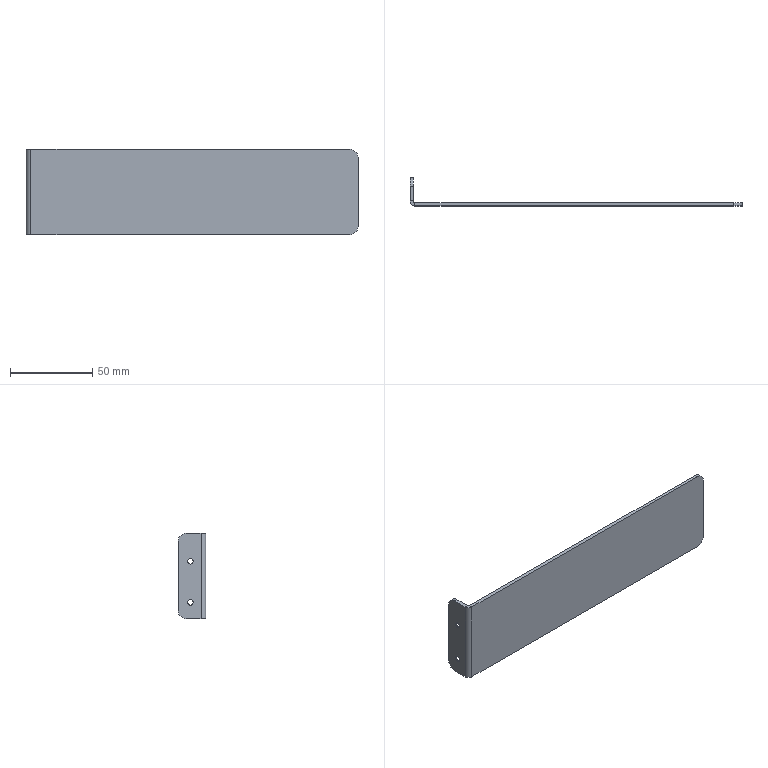Part | NX | features BREP 1 | 1 solid | 26 faces | box 202 x 17 x 52 mm | volume 22366 mm3 | plane 12 | cylinder 10 | cone 4 | commonest cylinder face diameters 3.4 x4 10 x4 2 x1 6 x1
STEP:
#1=CARTESIAN_POINT('',(-1.55,7.5,10.7));
#2=VERTEX_POINT('',#1);
#3=CARTESIAN_POINT('',(0.,7.5,12.25));
#4=VERTEX_POINT('',#3);
#5=CARTESIAN_POINT('',(0.,7.5,12.25));
#6=DIRECTION('',(0.7071,0.,0.7071));
#7=VECTOR('',#6,1000.);
#8=LINE('',#5,#7);
#9=EDGE_CURVE('',#2,#4,#8,.T.);
#10=ORIENTED_EDGE('',*,*,#9,.F.);
#11=CARTESIAN_POINT('',(-1.55,7.5,7.3));
#12=VERTEX_POINT('',#11);
#13=CARTESIAN_POINT('',(-1.55,7.5,9.));
#14=DIRECTION('',(1.,0.,0.));
#15=DIRECTION('',(0.,0.,-1.));
#16=AXIS2_PLACEMENT_3D('',#13,#14,#15);
#17=CIRCLE('',#16,1.7);
#18=EDGE_CURVE('',#12,#2,#17,.T.);
#19=ORIENTED_EDGE('',*,*,#18,.F.);
#20=CARTESIAN_POINT('',(0.,7.5,5.75));
#21=VERTEX_POINT('',#20);
#22=CARTESIAN_POINT('',(0.,7.5,5.75));
#23=DIRECTION('',(0.7071,0.,-0.7071));
#24=VECTOR('',#23,1000.);
#25=LINE('',#22,#24);
#26=EDGE_CURVE('',#12,#21,#25,.T.);
#27=ORIENTED_EDGE('',*,*,#26,.T.);
#28=CARTESIAN_POINT('',(0.,7.5,9.));
#29=DIRECTION('',(1.,0.,0.));
#30=DIRECTION('',(0.,0.,-1.));
#31=AXIS2_PLACEMENT_3D('',#28,#29,#30);
#32=CIRCLE('',#31,3.25);
#33=EDGE_CURVE('',#21,#4,#32,.T.);
#34=ORIENTED_EDGE('',*,*,#33,.T.);
#35=EDGE_LOOP('',(#10,#19,#27,#34));
#36=FACE_BOUND('',#35,.T.);
#37=CARTESIAN_POINT('',(0.,7.5,9.));
#38=DIRECTION('',(1.,0.,0.));
#39=DIRECTION('',(0.,0.,-1.));
#40=AXIS2_PLACEMENT_3D('',#37,#38,#39);
#41=CONICAL_SURFACE('',#40,3.25,0.7854);
#42=ADVANCED_FACE('',(#36),#41,.F.);
#43=CARTESIAN_POINT('',(-2.,7.5,10.7));
#44=VERTEX_POINT('',#43);
#45=CARTESIAN_POINT('',(0.,7.5,10.7));
#46=DIRECTION('',(1.,0.,0.));
#47=VECTOR('',#46,1000.);
#48=LINE('',#45,#47);
#49=EDGE_CURVE('',#44,#2,#48,.T.);
#50=ORIENTED_EDGE('',*,*,#49,.F.);
#51=CARTESIAN_POINT('',(-2.,7.5,7.3));
#52=VERTEX_POINT('',#51);
#53=CARTESIAN_POINT('',(-2.,7.5,9.));
#54=DIRECTION('',(1.,0.,0.));
#55=DIRECTION('',(0.,0.,-1.));
#56=AXIS2_PLACEMENT_3D('',#53,#54,#55);
#57=CIRCLE('',#56,1.7);
#58=EDGE_CURVE('',#52,#44,#57,.T.);
#59=ORIENTED_EDGE('',*,*,#58,.F.);
#60=CARTESIAN_POINT('',(0.,7.5,7.3));
#61=DIRECTION('',(1.,0.,0.));
#62=VECTOR('',#61,1000.);
#63=LINE('',#60,#62);
#64=EDGE_CURVE('',#52,#12,#63,.T.);
#65=ORIENTED_EDGE('',*,*,#64,.T.);
#66=ORIENTED_EDGE('',*,*,#18,.T.);
#67=EDGE_LOOP('',(#50,#59,#65,#66));
#68=FACE_BOUND('',#67,.T.);
#69=CARTESIAN_POINT('',(0.,7.5,9.));
#70=DIRECTION('',(1.,0.,0.));
#71=DIRECTION('',(0.,0.,-1.));
#72=AXIS2_PLACEMENT_3D('',#69,#70,#71);
#73=CYLINDRICAL_SURFACE('',#72,1.7);
#74=ADVANCED_FACE('',(#68),#73,.F.);
#75=CARTESIAN_POINT('',(-1.55,7.5,-14.3));
#76=VERTEX_POINT('',#75);
#77=CARTESIAN_POINT('',(0.,7.5,-12.75));
#78=VERTEX_POINT('',#77);
#79=CARTESIAN_POINT('',(0.,7.5,-12.75));
#80=DIRECTION('',(0.7071,0.,0.7071));
#81=VECTOR('',#80,1000.);
#82=LINE('',#79,#81);
#83=EDGE_CURVE('',#76,#78,#82,.T.);
#84=ORIENTED_EDGE('',*,*,#83,.F.);
#85=CARTESIAN_POINT('',(-1.55,7.5,-17.7));
#86=VERTEX_POINT('',#85);
#87=CARTESIAN_POINT('',(-1.55,7.5,-16.));
#88=DIRECTION('',(1.,0.,0.));
#89=DIRECTION('',(0.,0.,-1.));
#90=AXIS2_PLACEMENT_3D('',#87,#88,#89);
#91=CIRCLE('',#90,1.7);
#92=EDGE_CURVE('',#86,#76,#91,.T.);
#93=ORIENTED_EDGE('',*,*,#92,.F.);
#94=CARTESIAN_POINT('',(0.,7.5,-19.25));
#95=VERTEX_POINT('',#94);
#96=CARTESIAN_POINT('',(0.,7.5,-19.25));
#97=DIRECTION('',(0.7071,0.,-0.7071));
#98=VECTOR('',#97,1000.);
#99=LINE('',#96,#98);
#100=EDGE_CURVE('',#86,#95,#99,.T.);
#101=ORIENTED_EDGE('',*,*,#100,.T.);
#102=CARTESIAN_POINT('',(0.,7.5,-16.));
#103=DIRECTION('',(1.,0.,0.));
#104=DIRECTION('',(0.,0.,-1.));
#105=AXIS2_PLACEMENT_3D('',#102,#103,#104);
#106=CIRCLE('',#105,3.25);
#107=EDGE_CURVE('',#95,#78,#106,.T.);
#108=ORIENTED_EDGE('',*,*,#107,.T.);
#109=EDGE_LOOP('',(#84,#93,#101,#108));
#110=FACE_BOUND('',#109,.T.);
#111=CARTESIAN_POINT('',(0.,7.5,-16.));
#112=DIRECTION('',(1.,0.,0.));
#113=DIRECTION('',(0.,0.,-1.));
#114=AXIS2_PLACEMENT_3D('',#111,#112,#113);
#115=CONICAL_SURFACE('',#114,3.25,0.7854);
#116=ADVANCED_FACE('',(#110),#115,.F.);
#117=CARTESIAN_POINT('',(-2.,7.5,-14.3));
#118=VERTEX_POINT('',#117);
#119=CARTESIAN_POINT('',(0.,7.5,-14.3));
#120=DIRECTION('',(1.,0.,0.));
#121=VECTOR('',#120,1000.);
#122=LINE('',#119,#121);
#123=EDGE_CURVE('',#118,#76,#122,.T.);
#124=ORIENTED_EDGE('',*,*,#123,.F.);
#125=CARTESIAN_POINT('',(-2.,7.5,-17.7));
#126=VERTEX_POINT('',#125);
#127=CARTESIAN_POINT('',(-2.,7.5,-16.));
#128=DIRECTION('',(1.,0.,0.));
#129=DIRECTION('',(0.,0.,-1.));
#130=AXIS2_PLACEMENT_3D('',#127,#128,#129);
#131=CIRCLE('',#130,1.7);
#132=EDGE_CURVE('',#126,#118,#131,.T.);
#133=ORIENTED_EDGE('',*,*,#132,.F.);
#134=CARTESIAN_POINT('',(0.,7.5,-17.7));
#135=DIRECTION('',(1.,0.,0.));
#136=VECTOR('',#135,1000.);
#137=LINE('',#134,#136);
#138=EDGE_CURVE('',#126,#86,#137,.T.);
#139=ORIENTED_EDGE('',*,*,#138,.T.);
#140=ORIENTED_EDGE('',*,*,#92,.T.);
#141=EDGE_LOOP('',(#124,#133,#139,#140));
#142=FACE_BOUND('',#141,.T.);
#143=CARTESIAN_POINT('',(0.,7.5,-16.));
#144=DIRECTION('',(1.,0.,0.));
#145=DIRECTION('',(0.,0.,-1.));
#146=AXIS2_PLACEMENT_3D('',#143,#144,#145);
#147=CYLINDRICAL_SURFACE('',#146,1.7);
#148=ADVANCED_FACE('',(#142),#147,.F.);
#149=CARTESIAN_POINT('',(-2.,15.,-21.));
#150=VERTEX_POINT('',#149);
#151=CARTESIAN_POINT('',(-2.,10.,-26.));
#152=VERTEX_POINT('',#151);
#153=CARTESIAN_POINT('',(-2.,10.,-21.));
#154=DIRECTION('',(-1.,0.,0.));
#155=DIRECTION('',(0.,0.,-1.));
#156=AXIS2_PLACEMENT_3D('',#153,#154,#155);
#157=CIRCLE('',#156,5.);
#158=EDGE_CURVE('',#150,#152,#157,.T.);
#159=ORIENTED_EDGE('',*,*,#158,.F.);
#160=CARTESIAN_POINT('',(0.,15.,-21.));
#161=VERTEX_POINT('',#160);
#162=CARTESIAN_POINT('',(-2.,15.,-21.));
#163=DIRECTION('',(-1.,0.,0.));
#164=VECTOR('',#163,1000.);
#165=LINE('',#162,#164);
#166=EDGE_CURVE('',#161,#150,#165,.T.);
#167=ORIENTED_EDGE('',*,*,#166,.F.);
#168=CARTESIAN_POINT('',(0.,10.,-26.));
#169=VERTEX_POINT('',#168);
#170=CARTESIAN_POINT('',(0.,10.,-21.));
#171=DIRECTION('',(1.,0.,0.));
#172=DIRECTION('',(0.,0.,-1.));
#173=AXIS2_PLACEMENT_3D('',#170,#171,#172);
#174=CIRCLE('',#173,5.);
#175=EDGE_CURVE('',#169,#161,#174,.T.);
#176=ORIENTED_EDGE('',*,*,#175,.F.);
#177=CARTESIAN_POINT('',(1.,10.,-26.));
#178=DIRECTION('',(1.,0.,0.));
#179=VECTOR('',#178,1000.);
#180=LINE('',#177,#179);
#181=EDGE_CURVE('',#152,#169,#180,.T.);
#182=ORIENTED_EDGE('',*,*,#181,.F.);
#183=EDGE_LOOP('',(#159,#167,#176,#182));
#184=FACE_BOUND('',#183,.T.);
#185=CARTESIAN_POINT('',(1.,10.,-21.));
#186=DIRECTION('',(1.,0.,0.));
#187=DIRECTION('',(0.,0.,-1.));
#188=AXIS2_PLACEMENT_3D('',#185,#186,#187);
#189=CYLINDRICAL_SURFACE('',#188,5.);
#190=ADVANCED_FACE('',(#184),#189,.T.);
#191=CARTESIAN_POINT('',(-2.,10.,26.));
#192=VERTEX_POINT('',#191);
#193=CARTESIAN_POINT('',(-2.,15.,21.));
#194=VERTEX_POINT('',#193);
#195=CARTESIAN_POINT('',(-2.,10.,21.));
#196=DIRECTION('',(-1.,0.,0.));
#197=DIRECTION('',(0.,0.,-1.));
#198=AXIS2_PLACEMENT_3D('',#195,#196,#197);
#199=CIRCLE('',#198,5.);
#200=EDGE_CURVE('',#192,#194,#199,.T.);
#201=ORIENTED_EDGE('',*,*,#200,.F.);
#202=CARTESIAN_POINT('',(0.,10.,26.));
#203=VERTEX_POINT('',#202);
#204=CARTESIAN_POINT('',(-2.,10.,26.));
#205=DIRECTION('',(-1.,0.,0.));
#206=VECTOR('',#205,1000.);
#207=LINE('',#204,#206);
#208=EDGE_CURVE('',#203,#192,#207,.T.);
#209=ORIENTED_EDGE('',*,*,#208,.F.);
#210=CARTESIAN_POINT('',(0.,15.,21.));
#211=VERTEX_POINT('',#210);
#212=CARTESIAN_POINT('',(0.,10.,21.));
#213=DIRECTION('',(1.,0.,0.));
#214=DIRECTION('',(0.,0.,-1.));
#215=AXIS2_PLACEMENT_3D('',#212,#213,#214);
#216=CIRCLE('',#215,5.);
#217=EDGE_CURVE('',#211,#203,#216,.T.);
#218=ORIENTED_EDGE('',*,*,#217,.F.);
#219=CARTESIAN_POINT('',(0.,15.,21.));
#220=DIRECTION('',(1.,0.,0.));
#221=VECTOR('',#220,1000.);
#222=LINE('',#219,#221);
#223=EDGE_CURVE('',#194,#211,#222,.T.);
#224=ORIENTED_EDGE('',*,*,#223,.F.);
#225=EDGE_LOOP('',(#201,#209,#218,#224));
#226=FACE_BOUND('',#225,.T.);
#227=CARTESIAN_POINT('',(-2.,10.,21.));
#228=DIRECTION('',(-1.,0.,0.));
#229=DIRECTION('',(0.,0.,1.));
#230=AXIS2_PLACEMENT_3D('',#227,#228,#229);
#231=CYLINDRICAL_SURFACE('',#230,5.);
#232=ADVANCED_FACE('',(#226),#231,.T.);
#233=CARTESIAN_POINT('',(195.,0.,26.));
#234=VERTEX_POINT('',#233);
#235=CARTESIAN_POINT('',(200.,0.,21.));
#236=VERTEX_POINT('',#235);
#237=CARTESIAN_POINT('',(195.,0.,21.));
#238=DIRECTION('',(0.,1.,0.));
#239=DIRECTION('',(0.,0.,1.));
#240=AXIS2_PLACEMENT_3D('',#237,#238,#239);
#241=CIRCLE('',#240,5.);
#242=EDGE_CURVE('',#234,#236,#241,.T.);
#243=ORIENTED_EDGE('',*,*,#242,.F.);
#244=CARTESIAN_POINT('',(195.,-2.,26.));
#245=VERTEX_POINT('',#244);
#246=CARTESIAN_POINT('',(195.,1.,26.));
#247=DIRECTION('',(0.,1.,0.));
#248=VECTOR('',#247,1000.);
#249=LINE('',#246,#248);
#250=EDGE_CURVE('',#245,#234,#249,.T.);
#251=ORIENTED_EDGE('',*,*,#250,.F.);
#252=CARTESIAN_POINT('',(200.,-2.,21.));
#253=VERTEX_POINT('',#252);
#254=CARTESIAN_POINT('',(195.,-2.,21.));
#255=DIRECTION('',(0.,-1.,0.));
#256=DIRECTION('',(0.,0.,1.));
#257=AXIS2_PLACEMENT_3D('',#254,#255,#256);
#258=CIRCLE('',#257,5.);
#259=EDGE_CURVE('',#253,#245,#258,.T.);
#260=ORIENTED_EDGE('',*,*,#259,.F.);
#261=CARTESIAN_POINT('',(200.,0.,21.));
#262=DIRECTION('',(0.,-1.,0.));
#263=VECTOR('',#262,1000.);
#264=LINE('',#261,#263);
#265=EDGE_CURVE('',#236,#253,#264,.T.);
#266=ORIENTED_EDGE('',*,*,#265,.F.);
#267=EDGE_LOOP('',(#243,#251,#260,#266));
#268=FACE_BOUND('',#267,.T.);
#269=CARTESIAN_POINT('',(195.,0.,21.));
#270=DIRECTION('',(0.,-1.,0.));
#271=DIRECTION('',(0.,0.,-1.));
#272=AXIS2_PLACEMENT_3D('',#269,#270,#271);
#273=CYLINDRICAL_SURFACE('',#272,5.);
#274=ADVANCED_FACE('',(#268),#273,.T.);
#275=CARTESIAN_POINT('',(200.,0.,-21.));
#276=VERTEX_POINT('',#275);
#277=CARTESIAN_POINT('',(195.,0.,-26.));
#278=VERTEX_POINT('',#277);
#279=CARTESIAN_POINT('',(195.,0.,-21.));
#280=DIRECTION('',(0.,1.,0.));
#281=DIRECTION('',(0.,0.,1.));
#282=AXIS2_PLACEMENT_3D('',#279,#280,#281);
#283=CIRCLE('',#282,5.);
#284=EDGE_CURVE('',#276,#278,#283,.T.);
#285=ORIENTED_EDGE('',*,*,#284,.F.);
#286=CARTESIAN_POINT('',(200.,-2.,-21.));
#287=VERTEX_POINT('',#286);
#288=CARTESIAN_POINT('',(200.,0.,-21.));
#289=DIRECTION('',(0.,1.,0.));
#290=VECTOR('',#289,1000.);
#291=LINE('',#288,#290);
#292=EDGE_CURVE('',#287,#276,#291,.T.);
#293=ORIENTED_EDGE('',*,*,#292,.F.);
#294=CARTESIAN_POINT('',(195.,-2.,-26.));
#295=VERTEX_POINT('',#294);
#296=CARTESIAN_POINT('',(195.,-2.,-21.));
#297=DIRECTION('',(0.,-1.,0.));
#298=DIRECTION('',(0.,0.,1.));
#299=AXIS2_PLACEMENT_3D('',#296,#297,#298);
#300=CIRCLE('',#299,5.);
#301=EDGE_CURVE('',#295,#287,#300,.T.);
#302=ORIENTED_EDGE('',*,*,#301,.F.);
#303=CARTESIAN_POINT('',(195.,1.,-26.));
#304=DIRECTION('',(0.,-1.,0.));
#305=VECTOR('',#304,1000.);
#306=LINE('',#303,#305);
#307=EDGE_CURVE('',#278,#295,#306,.T.);
#308=ORIENTED_EDGE('',*,*,#307,.F.);
#309=EDGE_LOOP('',(#285,#293,#302,#308));
#310=FACE_BOUND('',#309,.T.);
#311=CARTESIAN_POINT('',(195.,1.,-21.));
#312=DIRECTION('',(0.,-1.,0.));
#313=DIRECTION('',(0.,0.,-1.));
#314=AXIS2_PLACEMENT_3D('',#311,#312,#313);
#315=CYLINDRICAL_SURFACE('',#314,5.);
#316=ADVANCED_FACE('',(#310),#315,.T.);
#317=CARTESIAN_POINT('',(1.,0.,-26.));
#318=VERTEX_POINT('',#317);
#319=CARTESIAN_POINT('',(0.,0.,-26.));
#320=DIRECTION('',(1.,0.,0.));
#321=VECTOR('',#320,1000.);
#322=LINE('',#319,#321);
#323=EDGE_CURVE('',#318,#278,#322,.T.);
#324=ORIENTED_EDGE('',*,*,#323,.T.);
#325=ORIENTED_EDGE('',*,*,#307,.T.);
#326=CARTESIAN_POINT('',(1.,-2.,-26.));
#327=VERTEX_POINT('',#326);
#328=CARTESIAN_POINT('',(0.,-2.,-26.));
#329=DIRECTION('',(1.,0.,0.));
#330=VECTOR('',#329,1000.);
#331=LINE('',#328,#330);
#332=EDGE_CURVE('',#327,#295,#331,.T.);
#333=ORIENTED_EDGE('',*,*,#332,.F.);
#334=CARTESIAN_POINT('',(1.,-2.,-26.));
#335=DIRECTION('',(0.,1.,0.));
#336=VECTOR('',#335,1000.);
#337=LINE('',#334,#336);
#338=EDGE_CURVE('',#327,#318,#337,.T.);
#339=ORIENTED_EDGE('',*,*,#338,.T.);
#340=EDGE_LOOP('',(#324,#325,#333,#339));
#341=FACE_BOUND('',#340,.T.);
#342=CARTESIAN_POINT('',(1.,1.,-26.));
#343=DIRECTION('',(0.,0.,-1.));
#344=DIRECTION('',(-1.,0.,0.));
#345=AXIS2_PLACEMENT_3D('',#342,#343,#344);
#346=PLANE('',#345);
#347=ADVANCED_FACE('',(#341),#346,.T.);
#348=CARTESIAN_POINT('',(0.,1.,26.));
#349=VERTEX_POINT('',#348);
#350=CARTESIAN_POINT('',(0.,15.,26.));
#351=DIRECTION('',(0.,-1.,0.));
#352=VECTOR('',#351,1000.);
#353=LINE('',#350,#352);
#354=EDGE_CURVE('',#203,#349,#353,.T.);
#355=ORIENTED_EDGE('',*,*,#354,.F.);
#356=ORIENTED_EDGE('',*,*,#208,.T.);
#357=CARTESIAN_POINT('',(-2.,1.,26.));
#358=VERTEX_POINT('',#357);
#359=CARTESIAN_POINT('',(-2.,15.,26.));
#360=DIRECTION('',(0.,-1.,0.));
#361=VECTOR('',#360,1000.);
#362=LINE('',#359,#361);
#363=EDGE_CURVE('',#192,#358,#362,.T.);
#364=ORIENTED_EDGE('',*,*,#363,.T.);
#365=CARTESIAN_POINT('',(-2.,1.,26.));
#366=DIRECTION('',(1.,0.,0.));
#367=VECTOR('',#366,1000.);
#368=LINE('',#365,#367);
#369=EDGE_CURVE('',#358,#349,#368,.T.);
#370=ORIENTED_EDGE('',*,*,#369,.T.);
#371=EDGE_LOOP('',(#355,#356,#364,#370));
#372=FACE_BOUND('',#371,.T.);
#373=CARTESIAN_POINT('',(1.,1.,26.));
#374=DIRECTION('',(0.,0.,-1.));
#375=DIRECTION('',(-1.,0.,0.));
#376=AXIS2_PLACEMENT_3D('',#373,#374,#375);
#377=PLANE('',#376);
#378=ADVANCED_FACE('',(#372),#377,.F.);
#379=CARTESIAN_POINT('',(-2.,1.,-26.));
#380=VERTEX_POINT('',#379);
#381=CARTESIAN_POINT('',(1.,1.,-26.));
#382=DIRECTION('',(0.,0.,1.));
#383=DIRECTION('',(1.,0.,0.));
#384=AXIS2_PLACEMENT_3D('',#381,#382,#383);
#385=CIRCLE('',#384,3.);
#386=EDGE_CURVE('',#380,#327,#385,.T.);
#387=ORIENTED_EDGE('',*,*,#386,.T.);
#388=CARTESIAN_POINT('',(1.,-2.,26.));
#389=VERTEX_POINT('',#388);
#390=CARTESIAN_POINT('',(1.,-2.,26.));
#391=DIRECTION('',(0.,0.,-1.));
#392=VECTOR('',#391,1000.);
#393=LINE('',#390,#392);
#394=EDGE_CURVE('',#389,#327,#393,.T.);
#395=ORIENTED_EDGE('',*,*,#394,.F.);
#396=CARTESIAN_POINT('',(1.,1.,26.));
#397=DIRECTION('',(0.,0.,1.));
#398=DIRECTION('',(1.,0.,0.));
#399=AXIS2_PLACEMENT_3D('',#396,#397,#398);
#400=CIRCLE('',#399,3.);
#401=EDGE_CURVE('',#358,#389,#400,.T.);
#402=ORIENTED_EDGE('',*,*,#401,.F.);
#403=CARTESIAN_POINT('',(-2.,1.,26.));
#404=DIRECTION('',(0.,0.,-1.));
#405=VECTOR('',#404,1000.);
#406=LINE('',#403,#405);
#407=EDGE_CURVE('',#358,#380,#406,.T.);
#408=ORIENTED_EDGE('',*,*,#407,.T.);
#409=EDGE_LOOP('',(#387,#395,#402,#408));
#410=FACE_BOUND('',#409,.T.);
#411=CARTESIAN_POINT('',(1.,1.,26.));
#412=DIRECTION('',(0.,0.,-1.));
#413=DIRECTION('',(-1.,0.,0.));
#414=AXIS2_PLACEMENT_3D('',#411,#412,#413);
#415=CYLINDRICAL_SURFACE('',#414,3.);
#416=ADVANCED_FACE('',(#410),#415,.T.);
#417=ORIENTED_EDGE('',*,*,#363,.F.);
#418=ORIENTED_EDGE('',*,*,#200,.T.);
#419=CARTESIAN_POINT('',(-2.,15.,26.));
#420=DIRECTION('',(0.,0.,-1.));
#421=VECTOR('',#420,1000.);
#422=LINE('',#419,#421);
#423=EDGE_CURVE('',#194,#150,#422,.T.);
#424=ORIENTED_EDGE('',*,*,#423,.T.);
#425=ORIENTED_EDGE('',*,*,#158,.T.);
#426=CARTESIAN_POINT('',(-2.,15.,-26.));
#427=DIRECTION('',(0.,-1.,0.));
#428=VECTOR('',#427,1000.);
#429=LINE('',#426,#428);
#430=EDGE_CURVE('',#152,#380,#429,.T.);
#431=ORIENTED_EDGE('',*,*,#430,.T.);
#432=ORIENTED_EDGE('',*,*,#407,.F.);
#433=EDGE_LOOP('',(#417,#418,#424,#425,#431,#432));
#434=FACE_BOUND('',#433,.T.);
#435=ORIENTED_EDGE('',*,*,#132,.T.);
#436=CARTESIAN_POINT('',(-2.,7.5,-16.));
#437=DIRECTION('',(1.,0.,0.));
#438=DIRECTION('',(0.,0.,-1.));
#439=AXIS2_PLACEMENT_3D('',#436,#437,#438);
#440=CIRCLE('',#439,1.7);
#441=EDGE_CURVE('',#118,#126,#440,.T.);
#442=ORIENTED_EDGE('',*,*,#441,.T.);
#443=EDGE_LOOP('',(#435,#442));
#444=FACE_BOUND('',#443,.T.);
#445=ORIENTED_EDGE('',*,*,#58,.T.);
#446=CARTESIAN_POINT('',(-2.,7.5,9.));
#447=DIRECTION('',(1.,0.,0.));
#448=DIRECTION('',(0.,0.,-1.));
#449=AXIS2_PLACEMENT_3D('',#446,#447,#448);
#450=CIRCLE('',#449,1.7);
#451=EDGE_CURVE('',#44,#52,#450,.T.);
#452=ORIENTED_EDGE('',*,*,#451,.T.);
#453=EDGE_LOOP('',(#445,#452));
#454=FACE_BOUND('',#453,.T.);
#455=CARTESIAN_POINT('',(-2.,15.,26.));
#456=DIRECTION('',(1.,0.,0.));
#457=DIRECTION('',(0.,0.,-1.));
#458=AXIS2_PLACEMENT_3D('',#455,#456,#457);
#459=PLANE('',#458);
#460=ADVANCED_FACE('',(#434,#444,#454),#459,.F.);
#461=ORIENTED_EDGE('',*,*,#423,.F.);
#462=ORIENTED_EDGE('',*,*,#223,.T.);
#463=CARTESIAN_POINT('',(0.,15.,26.));
#464=DIRECTION('',(0.,0.,-1.));
#465=VECTOR('',#464,1000.);
#466=LINE('',#463,#465);
#467=EDGE_CURVE('',#211,#161,#466,.T.);
#468=ORIENTED_EDGE('',*,*,#467,.T.);
#469=ORIENTED_EDGE('',*,*,#166,.T.);
#470=EDGE_LOOP('',(#461,#462,#468,#469));
#471=FACE_BOUND('',#470,.T.);
#472=CARTESIAN_POINT('',(-2.,15.,26.));
#473=DIRECTION('',(0.,1.,0.));
#474=DIRECTION('',(0.,0.,1.));
#475=AXIS2_PLACEMENT_3D('',#472,#473,#474);
#476=PLANE('',#475);
#477=ADVANCED_FACE('',(#471),#476,.T.);
#478=ORIENTED_EDGE('',*,*,#467,.F.);
#479=ORIENTED_EDGE('',*,*,#217,.T.);
#480=ORIENTED_EDGE('',*,*,#354,.T.);
#481=CARTESIAN_POINT('',(0.,1.,-26.));
#482=VERTEX_POINT('',#481);
#483=CARTESIAN_POINT('',(0.,1.,26.));
#484=DIRECTION('',(0.,0.,-1.));
#485=VECTOR('',#484,1000.);
#486=LINE('',#483,#485);
#487=EDGE_CURVE('',#349,#482,#486,.T.);
#488=ORIENTED_EDGE('',*,*,#487,.T.);
#489=CARTESIAN_POINT('',(0.,15.,-26.));
#490=DIRECTION('',(0.,-1.,0.));
#491=VECTOR('',#490,1000.);
#492=LINE('',#489,#491);
#493=EDGE_CURVE('',#169,#482,#492,.T.);
#494=ORIENTED_EDGE('',*,*,#493,.F.);
#495=ORIENTED_EDGE('',*,*,#175,.T.);
#496=EDGE_LOOP('',(#478,#479,#480,#488,#494,#495));
#497=FACE_BOUND('',#496,.T.);
#498=ORIENTED_EDGE('',*,*,#107,.F.);
#499=CARTESIAN_POINT('',(0.,7.5,-16.));
#500=DIRECTION('',(1.,0.,0.));
#501=DIRECTION('',(0.,0.,-1.));
#502=AXIS2_PLACEMENT_3D('',#499,#500,#501);
#503=CIRCLE('',#502,3.25);
#504=EDGE_CURVE('',#78,#95,#503,.T.);
#505=ORIENTED_EDGE('',*,*,#504,.F.);
#506=EDGE_LOOP('',(#498,#505));
#507=FACE_BOUND('',#506,.T.);
#508=ORIENTED_EDGE('',*,*,#33,.F.);
#509=CARTESIAN_POINT('',(0.,7.5,9.));
#510=DIRECTION('',(1.,0.,0.));
#511=DIRECTION('',(0.,0.,-1.));
#512=AXIS2_PLACEMENT_3D('',#509,#510,#511);
#513=CIRCLE('',#512,3.25);
#514=EDGE_CURVE('',#4,#21,#513,.T.);
#515=ORIENTED_EDGE('',*,*,#514,.F.);
#516=EDGE_LOOP('',(#508,#515));
#517=FACE_BOUND('',#516,.T.);
#518=CARTESIAN_POINT('',(0.,15.,26.));
#519=DIRECTION('',(1.,0.,0.));
#520=DIRECTION('',(0.,0.,-1.));
#521=AXIS2_PLACEMENT_3D('',#518,#519,#520);
#522=PLANE('',#521);
#523=ADVANCED_FACE('',(#497,#507,#517),#522,.T.);
#524=CARTESIAN_POINT('',(1.,1.,-26.));
#525=DIRECTION('',(0.,0.,1.));
#526=DIRECTION('',(-1.,0.,0.));
#527=AXIS2_PLACEMENT_3D('',#524,#525,#526);
#528=CIRCLE('',#527,1.);
#529=EDGE_CURVE('',#482,#318,#528,.T.);
#530=ORIENTED_EDGE('',*,*,#529,.F.);
#531=ORIENTED_EDGE('',*,*,#487,.F.);
#532=CARTESIAN_POINT('',(1.,0.,26.));
#533=VERTEX_POINT('',#532);
#534=CARTESIAN_POINT('',(1.,1.,26.));
#535=DIRECTION('',(0.,0.,1.));
#536=DIRECTION('',(-1.,0.,0.));
#537=AXIS2_PLACEMENT_3D('',#534,#535,#536);
#538=CIRCLE('',#537,1.);
#539=EDGE_CURVE('',#349,#533,#538,.T.);
#540=ORIENTED_EDGE('',*,*,#539,.T.);
#541=CARTESIAN_POINT('',(1.,0.,26.));
#542=DIRECTION('',(0.,0.,-1.));
#543=VECTOR('',#542,1000.);
#544=LINE('',#541,#543);
#545=EDGE_CURVE('',#533,#318,#544,.T.);
#546=ORIENTED_EDGE('',*,*,#545,.T.);
#547=EDGE_LOOP('',(#530,#531,#540,#546));
#548=FACE_BOUND('',#547,.T.);
#549=CARTESIAN_POINT('',(1.,1.,26.));
#550=DIRECTION('',(0.,0.,-1.));
#551=DIRECTION('',(-1.,0.,0.));
#552=AXIS2_PLACEMENT_3D('',#549,#550,#551);
#553=CYLINDRICAL_SURFACE('',#552,1.);
#554=ADVANCED_FACE('',(#548),#553,.F.);
#555=CARTESIAN_POINT('',(200.,0.,26.));
#556=DIRECTION('',(0.,0.,-1.));
#557=VECTOR('',#556,1000.);
#558=LINE('',#555,#557);
#559=EDGE_CURVE('',#236,#276,#558,.T.);
#560=ORIENTED_EDGE('',*,*,#559,.T.);
#561=ORIENTED_EDGE('',*,*,#284,.T.);
#562=ORIENTED_EDGE('',*,*,#323,.F.);
#563=ORIENTED_EDGE('',*,*,#545,.F.);
#564=CARTESIAN_POINT('',(0.,0.,26.));
#565=DIRECTION('',(1.,0.,0.));
#566=VECTOR('',#565,1000.);
#567=LINE('',#564,#566);
#568=EDGE_CURVE('',#533,#234,#567,.T.);
#569=ORIENTED_EDGE('',*,*,#568,.T.);
#570=ORIENTED_EDGE('',*,*,#242,.T.);
#571=EDGE_LOOP('',(#560,#561,#562,#563,#569,#570));
#572=FACE_BOUND('',#571,.T.);
#573=CARTESIAN_POINT('',(0.,0.,26.));
#574=DIRECTION('',(0.,1.,0.));
#575=DIRECTION('',(0.,0.,1.));
#576=AXIS2_PLACEMENT_3D('',#573,#574,#575);
#577=PLANE('',#576);
#578=ADVANCED_FACE('',(#572),#577,.T.);
#579=CARTESIAN_POINT('',(200.,-2.,26.));
#580=DIRECTION('',(0.,0.,-1.));
#581=VECTOR('',#580,1000.);
#582=LINE('',#579,#581);
#583=EDGE_CURVE('',#253,#287,#582,.T.);
#584=ORIENTED_EDGE('',*,*,#583,.T.);
#585=ORIENTED_EDGE('',*,*,#292,.T.);
#586=ORIENTED_EDGE('',*,*,#559,.F.);
#587=ORIENTED_EDGE('',*,*,#265,.T.);
#588=EDGE_LOOP('',(#584,#585,#586,#587));
#589=FACE_BOUND('',#588,.T.);
#590=CARTESIAN_POINT('',(200.,0.,26.));
#591=DIRECTION('',(1.,0.,0.));
#592=DIRECTION('',(0.,0.,-1.));
#593=AXIS2_PLACEMENT_3D('',#590,#591,#592);
#594=PLANE('',#593);
#595=ADVANCED_FACE('',(#589),#594,.T.);
#596=ORIENTED_EDGE('',*,*,#332,.T.);
#597=ORIENTED_EDGE('',*,*,#301,.T.);
#598=ORIENTED_EDGE('',*,*,#583,.F.);
#599=ORIENTED_EDGE('',*,*,#259,.T.);
#600=CARTESIAN_POINT('',(0.,-2.,26.));
#601=DIRECTION('',(1.,0.,0.));
#602=VECTOR('',#601,1000.);
#603=LINE('',#600,#602);
#604=EDGE_CURVE('',#389,#245,#603,.T.);
#605=ORIENTED_EDGE('',*,*,#604,.F.);
#606=ORIENTED_EDGE('',*,*,#394,.T.);
#607=EDGE_LOOP('',(#596,#597,#598,#599,#605,#606));
#608=FACE_BOUND('',#607,.T.);
#609=CARTESIAN_POINT('',(0.,-2.,26.));
#610=DIRECTION('',(0.,1.,0.));
#611=DIRECTION('',(0.,0.,1.));
#612=AXIS2_PLACEMENT_3D('',#609,#610,#611);
#613=PLANE('',#612);
#614=ADVANCED_FACE('',(#608),#613,.F.);
#615=ORIENTED_EDGE('',*,*,#430,.F.);
#616=ORIENTED_EDGE('',*,*,#181,.T.);
#617=ORIENTED_EDGE('',*,*,#493,.T.);
#618=CARTESIAN_POINT('',(0.,1.,-26.));
#619=DIRECTION('',(-1.,0.,0.));
#620=VECTOR('',#619,1000.);
#621=LINE('',#618,#620);
#622=EDGE_CURVE('',#482,#380,#621,.T.);
#623=ORIENTED_EDGE('',*,*,#622,.T.);
#624=EDGE_LOOP('',(#615,#616,#617,#623));
#625=FACE_BOUND('',#624,.T.);
#626=CARTESIAN_POINT('',(1.,-2.,-26.));
#627=DIRECTION('',(0.,0.,-1.));
#628=DIRECTION('',(-1.,0.,0.));
#629=AXIS2_PLACEMENT_3D('',#626,#627,#628);
#630=PLANE('',#629);
#631=ADVANCED_FACE('',(#625),#630,.T.);
#632=ORIENTED_EDGE('',*,*,#622,.F.);
#633=ORIENTED_EDGE('',*,*,#529,.T.);
#634=ORIENTED_EDGE('',*,*,#338,.F.);
#635=ORIENTED_EDGE('',*,*,#386,.F.);
#636=EDGE_LOOP('',(#632,#633,#634,#635));
#637=FACE_BOUND('',#636,.T.);
#638=CARTESIAN_POINT('',(0.,1.,-26.));
#639=DIRECTION('',(0.,0.,-1.));
#640=DIRECTION('',(-1.,0.,0.));
#641=AXIS2_PLACEMENT_3D('',#638,#639,#640);
#642=PLANE('',#641);
#643=ADVANCED_FACE('',(#637),#642,.T.);
#644=ORIENTED_EDGE('',*,*,#604,.T.);
#645=ORIENTED_EDGE('',*,*,#250,.T.);
#646=ORIENTED_EDGE('',*,*,#568,.F.);
#647=CARTESIAN_POINT('',(1.,0.,26.));
#648=DIRECTION('',(0.,-1.,0.));
#649=VECTOR('',#648,1000.);
#650=LINE('',#647,#649);
#651=EDGE_CURVE('',#533,#389,#650,.T.);
#652=ORIENTED_EDGE('',*,*,#651,.T.);
#653=EDGE_LOOP('',(#644,#645,#646,#652));
#654=FACE_BOUND('',#653,.T.);
#655=CARTESIAN_POINT('',(-2.,1.,26.));
#656=DIRECTION('',(0.,0.,1.));
#657=DIRECTION('',(1.,0.,0.));
#658=AXIS2_PLACEMENT_3D('',#655,#656,#657);
#659=PLANE('',#658);
#660=ADVANCED_FACE('',(#654),#659,.T.);
#661=ORIENTED_EDGE('',*,*,#651,.F.);
#662=ORIENTED_EDGE('',*,*,#539,.F.);
#663=ORIENTED_EDGE('',*,*,#369,.F.);
#664=ORIENTED_EDGE('',*,*,#401,.T.);
#665=EDGE_LOOP('',(#661,#662,#663,#664));
#666=FACE_BOUND('',#665,.T.);
#667=CARTESIAN_POINT('',(1.,0.,26.));
#668=DIRECTION('',(0.,0.,1.));
#669=DIRECTION('',(1.,0.,0.));
#670=AXIS2_PLACEMENT_3D('',#667,#668,#669);
#671=PLANE('',#670);
#672=ADVANCED_FACE('',(#666),#671,.T.);
#673=ORIENTED_EDGE('',*,*,#441,.F.);
#674=ORIENTED_EDGE('',*,*,#123,.T.);
#675=CARTESIAN_POINT('',(-1.55,7.5,-16.));
#676=DIRECTION('',(1.,0.,0.));
#677=DIRECTION('',(0.,0.,-1.));
#678=AXIS2_PLACEMENT_3D('',#675,#676,#677);
#679=CIRCLE('',#678,1.7);
#680=EDGE_CURVE('',#76,#86,#679,.T.);
#681=ORIENTED_EDGE('',*,*,#680,.T.);
#682=ORIENTED_EDGE('',*,*,#138,.F.);
#683=EDGE_LOOP('',(#673,#674,#681,#682));
#684=FACE_BOUND('',#683,.T.);
#685=CARTESIAN_POINT('',(0.,7.5,-16.));
#686=DIRECTION('',(1.,0.,0.));
#687=DIRECTION('',(0.,0.,-1.));
#688=AXIS2_PLACEMENT_3D('',#685,#686,#687);
#689=CYLINDRICAL_SURFACE('',#688,1.7);
#690=ADVANCED_FACE('',(#684),#689,.F.);
#691=ORIENTED_EDGE('',*,*,#680,.F.);
#692=ORIENTED_EDGE('',*,*,#83,.T.);
#693=ORIENTED_EDGE('',*,*,#504,.T.);
#694=ORIENTED_EDGE('',*,*,#100,.F.);
#695=EDGE_LOOP('',(#691,#692,#693,#694));
#696=FACE_BOUND('',#695,.T.);
#697=CARTESIAN_POINT('',(0.,7.5,-16.));
#698=DIRECTION('',(1.,0.,0.));
#699=DIRECTION('',(0.,0.,-1.));
#700=AXIS2_PLACEMENT_3D('',#697,#698,#699);
#701=CONICAL_SURFACE('',#700,3.25,0.7854);
#702=ADVANCED_FACE('',(#696),#701,.F.);
#703=ORIENTED_EDGE('',*,*,#451,.F.);
#704=ORIENTED_EDGE('',*,*,#49,.T.);
#705=CARTESIAN_POINT('',(-1.55,7.5,9.));
#706=DIRECTION('',(1.,0.,0.));
#707=DIRECTION('',(0.,0.,-1.));
#708=AXIS2_PLACEMENT_3D('',#705,#706,#707);
#709=CIRCLE('',#708,1.7);
#710=EDGE_CURVE('',#2,#12,#709,.T.);
#711=ORIENTED_EDGE('',*,*,#710,.T.);
#712=ORIENTED_EDGE('',*,*,#64,.F.);
#713=EDGE_LOOP('',(#703,#704,#711,#712));
#714=FACE_BOUND('',#713,.T.);
#715=CARTESIAN_POINT('',(0.,7.5,9.));
#716=DIRECTION('',(1.,0.,0.));
#717=DIRECTION('',(0.,0.,-1.));
#718=AXIS2_PLACEMENT_3D('',#715,#716,#717);
#719=CYLINDRICAL_SURFACE('',#718,1.7);
#720=ADVANCED_FACE('',(#714),#719,.F.);
#721=ORIENTED_EDGE('',*,*,#710,.F.);
#722=ORIENTED_EDGE('',*,*,#9,.T.);
#723=ORIENTED_EDGE('',*,*,#514,.T.);
#724=ORIENTED_EDGE('',*,*,#26,.F.);
#725=EDGE_LOOP('',(#721,#722,#723,#724));
#726=FACE_BOUND('',#725,.T.);
#727=CARTESIAN_POINT('',(0.,7.5,9.));
#728=DIRECTION('',(1.,0.,0.));
#729=DIRECTION('',(0.,0.,-1.));
#730=AXIS2_PLACEMENT_3D('',#727,#728,#729);
#731=CONICAL_SURFACE('',#730,3.25,0.7854);
#732=ADVANCED_FACE('',(#726),#731,.F.);
#733=CLOSED_SHELL('',(#42,#74,#116,#148,#190,#232,#274,#316,#347,#378,#416,#460,#477,#523,#554,#578,#595,#614,#631,#643,#660,#672,#690,#702,#720,#732));
#734=MANIFOLD_SOLID_BREP('',#733);
#735=(LENGTH_UNIT()NAMED_UNIT(*)SI_UNIT(.MILLI.,.METRE.));
#736=UNCERTAINTY_MEASURE_WITH_UNIT(LENGTH_MEASURE(0.00001),#735,'','');
#737=(NAMED_UNIT(*)PLANE_ANGLE_UNIT()SI_UNIT($,.RADIAN.));
#738=(NAMED_UNIT(*)SI_UNIT($,.STERADIAN.)SOLID_ANGLE_UNIT());
#739=(GEOMETRIC_REPRESENTATION_CONTEXT(3)GLOBAL_UNCERTAINTY_ASSIGNED_CONTEXT((#736))GLOBAL_UNIT_ASSIGNED_CONTEXT((#735,#737,#738))REPRESENTATION_CONTEXT('',''));
#740=ADVANCED_BREP_SHAPE_REPRESENTATION('',(#734),#739);